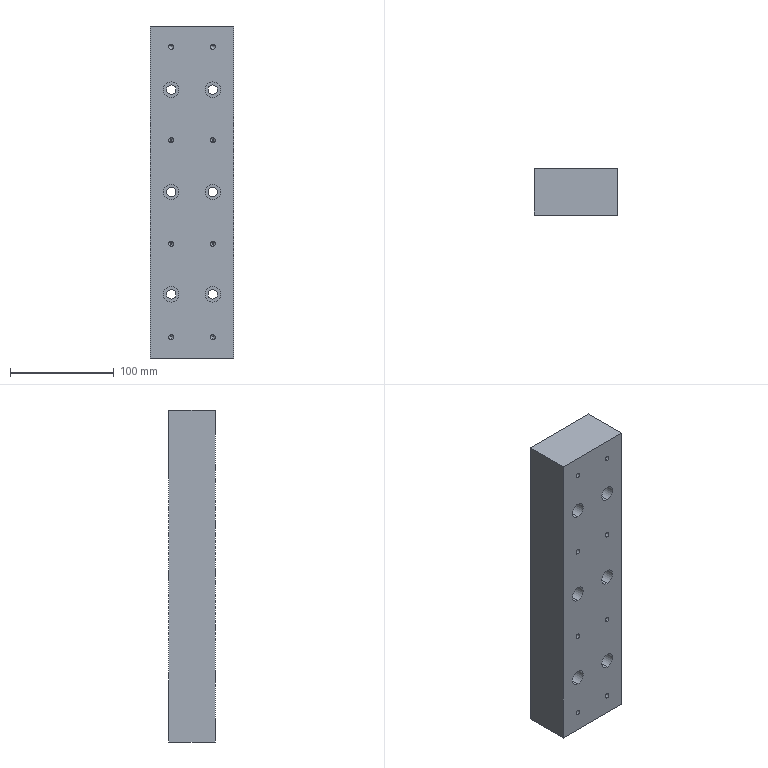Part | SolidWorks | features BaseBody 1 | 1 solid | 68 faces | box 80 x 45 x 320 mm | volume 1113853 mm3 | cylinder 40 | cone 16 | plane 12 | commonest cylinder face diameters 5 x16 9 x12 15 x12